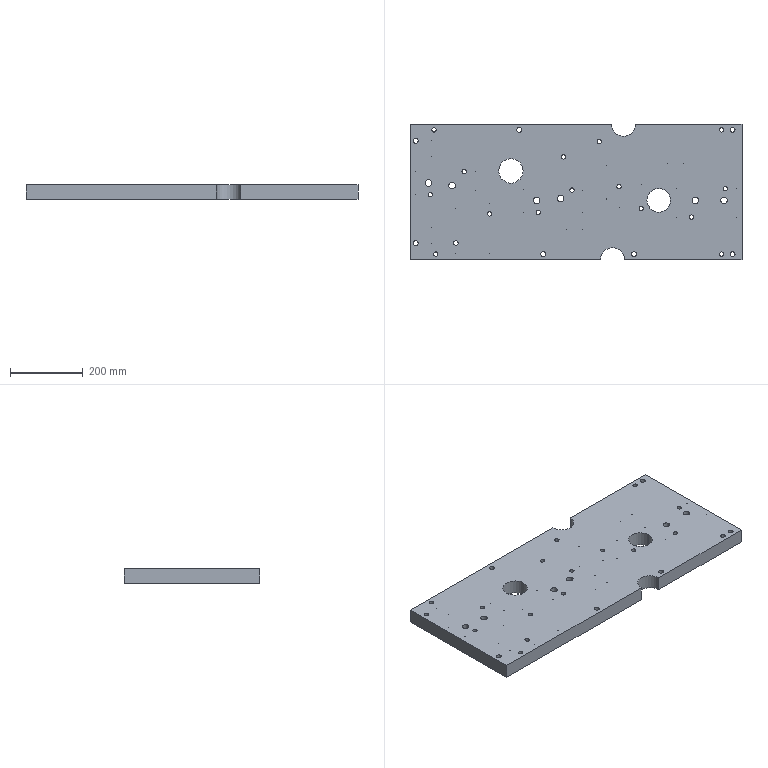Part | STEP file | lll_id2962_x_t | 1 solid | 142 faces | box 914 x 374 x 40 mm | volume 12947388 mm3 | cylinder 85 | cone 42 | plane 15 | commonest cylinder face diameters 10.506 x30 12 x16 13.509 x7 20.007 x7 10.505 x6 18 x6